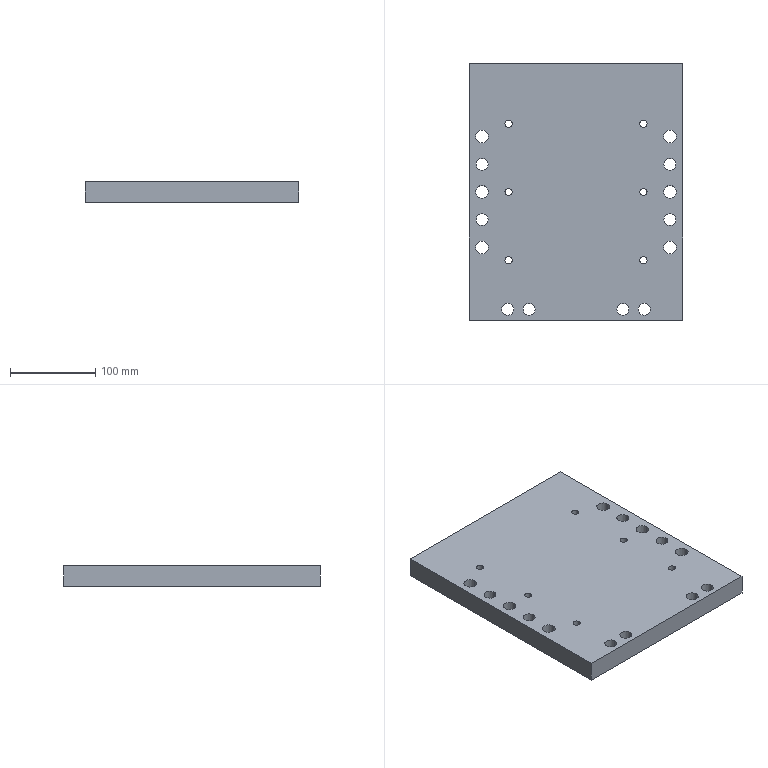Part | STEP file | MAT TRUOT DAU BUA KHONG LOGO | 1 solid | 46 faces | box 250 x 300 x 24 mm | volume 1737062 mm3 | cylinder 40 | plane 6 | commonest cylinder face diameters 14 x16 8.376 x12 15 x12